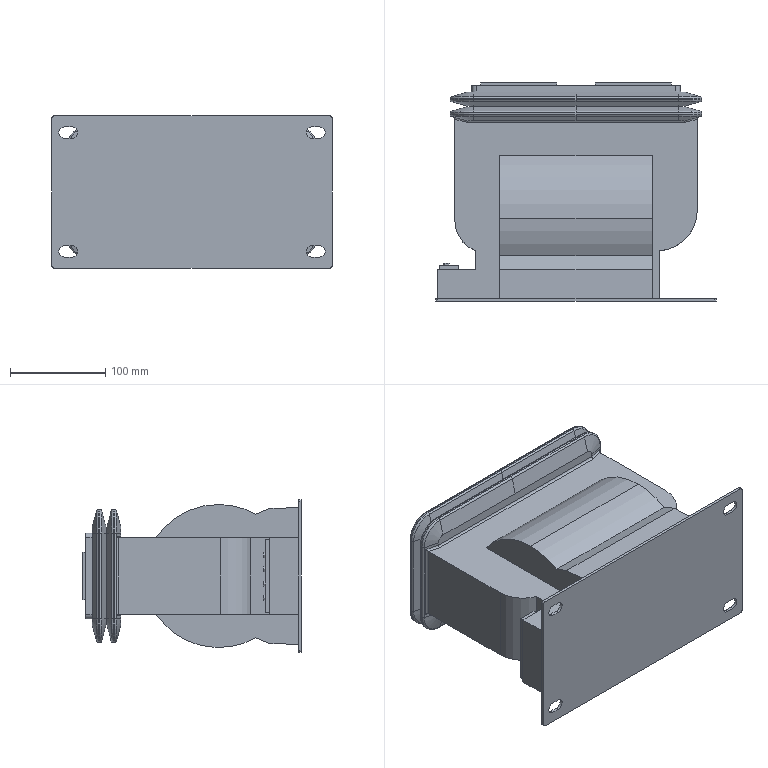Part | STEP file | Current transformer LZZJ9-10Q | 1 solid | 223 faces | box 295 x 230 x 160 mm | volume 6235515 mm3 | plane 113 | cylinder 70 | torus 24 | cone 16 | commonest cylinder face diameters 4 x32 12 x16 50 x8 0.2 x5 10 x4 158.915 x3